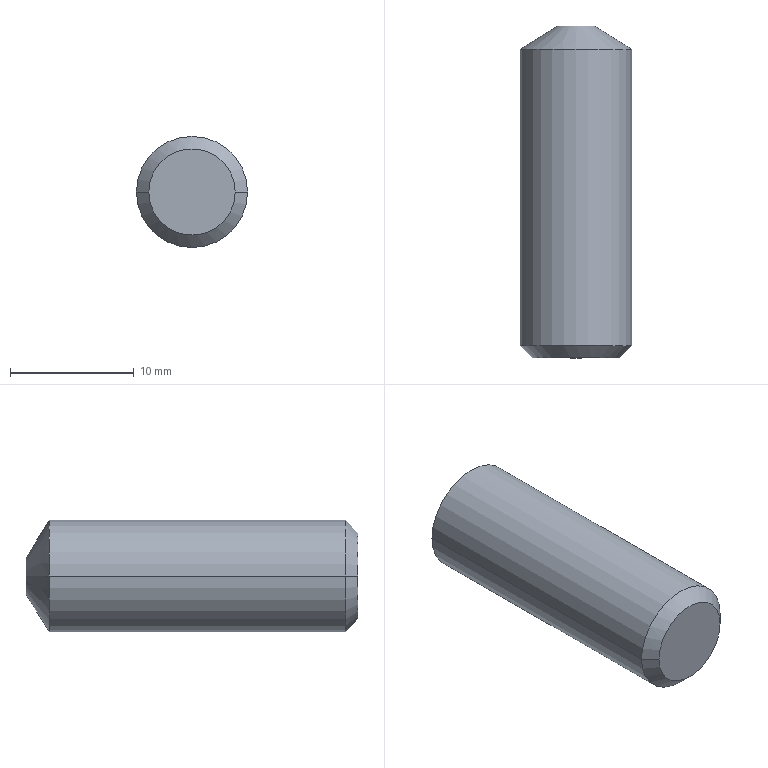Part | SolidWorks | features Chamfer 1, Revolution 1 | 1 solid | 8 faces | box 9 x 26.875 x 9 mm | volume 1635 mm3 | cone 4 | cylinder 2 | plane 2 | commonest cylinder face diameters 9 x2
STEP:
#1=CARTESIAN_POINT('',(3.5,0.,0.));
#2=VERTEX_POINT('',#1);
#3=CARTESIAN_POINT('',(-3.5,0.,0.));
#4=VERTEX_POINT('',#3);
#5=CARTESIAN_POINT('',(0.,0.,0.));
#6=DIRECTION('',(0.,-1.,0.));
#7=DIRECTION('',(1.,0.,0.));
#8=AXIS2_PLACEMENT_3D('',#5,#6,#7);
#9=CIRCLE('',#8,3.5);
#10=EDGE_CURVE('',#2,#4,#9,.T.);
#11=ORIENTED_EDGE('',*,*,#10,.F.);
#12=CARTESIAN_POINT('',(4.5,1.,0.));
#13=VERTEX_POINT('',#12);
#14=CARTESIAN_POINT('',(3.5,0.,0.));
#15=DIRECTION('',(0.7071,0.7071,0.));
#16=VECTOR('',#15,1000.);
#17=LINE('',#14,#16);
#18=EDGE_CURVE('',#2,#13,#17,.T.);
#19=ORIENTED_EDGE('',*,*,#18,.T.);
#20=CARTESIAN_POINT('',(-4.5,1.,0.));
#21=VERTEX_POINT('',#20);
#22=CARTESIAN_POINT('',(0.,1.,0.));
#23=DIRECTION('',(0.,1.,0.));
#24=DIRECTION('',(1.,0.,0.));
#25=AXIS2_PLACEMENT_3D('',#22,#23,#24);
#26=CIRCLE('',#25,4.5);
#27=EDGE_CURVE('',#21,#13,#26,.T.);
#28=ORIENTED_EDGE('',*,*,#27,.F.);
#29=CARTESIAN_POINT('',(-3.5,0.,0.));
#30=DIRECTION('',(-0.7071,0.7071,0.));
#31=VECTOR('',#30,1000.);
#32=LINE('',#29,#31);
#33=EDGE_CURVE('',#4,#21,#32,.T.);
#34=ORIENTED_EDGE('',*,*,#33,.F.);
#35=EDGE_LOOP('',(#11,#19,#28,#34));
#36=FACE_OUTER_BOUND('',#35,.T.);
#37=CARTESIAN_POINT('',(0.,0.,0.));
#38=DIRECTION('',(0.,1.,0.));
#39=DIRECTION('',(-1.,0.,0.));
#40=AXIS2_PLACEMENT_3D('',#37,#38,#39);
#41=CONICAL_SURFACE('',#40,3.5,0.7854);
#42=ADVANCED_FACE('',(#36),#41,.T.);
#43=CARTESIAN_POINT('',(4.5,25.,0.));
#44=VERTEX_POINT('',#43);
#45=CARTESIAN_POINT('',(-4.5,25.,0.));
#46=VERTEX_POINT('',#45);
#47=CARTESIAN_POINT('',(0.,25.,0.));
#48=DIRECTION('',(0.,-1.,0.));
#49=DIRECTION('',(1.,0.,0.));
#50=AXIS2_PLACEMENT_3D('',#47,#48,#49);
#51=CIRCLE('',#50,4.5);
#52=EDGE_CURVE('',#44,#46,#51,.T.);
#53=ORIENTED_EDGE('',*,*,#52,.T.);
#54=CARTESIAN_POINT('',(-4.5,0.,0.));
#55=DIRECTION('',(0.,-1.,0.));
#56=VECTOR('',#55,1000.);
#57=LINE('',#54,#56);
#58=EDGE_CURVE('',#46,#21,#57,.T.);
#59=ORIENTED_EDGE('',*,*,#58,.T.);
#60=ORIENTED_EDGE('',*,*,#27,.T.);
#61=CARTESIAN_POINT('',(4.5,0.,0.));
#62=DIRECTION('',(0.,-1.,0.));
#63=VECTOR('',#62,1000.);
#64=LINE('',#61,#63);
#65=EDGE_CURVE('',#44,#13,#64,.T.);
#66=ORIENTED_EDGE('',*,*,#65,.F.);
#67=EDGE_LOOP('',(#53,#59,#60,#66));
#68=FACE_OUTER_BOUND('',#67,.T.);
#69=CARTESIAN_POINT('',(0.,0.,0.));
#70=DIRECTION('',(0.,-1.,0.));
#71=DIRECTION('',(1.,0.,0.));
#72=AXIS2_PLACEMENT_3D('',#69,#70,#71);
#73=CYLINDRICAL_SURFACE('',#72,4.5);
#74=ADVANCED_FACE('',(#68),#73,.T.);
#75=CARTESIAN_POINT('',(1.5,26.875,0.));
#76=VERTEX_POINT('',#75);
#77=CARTESIAN_POINT('',(-1.5,26.875,0.));
#78=VERTEX_POINT('',#77);
#79=CARTESIAN_POINT('',(0.,26.875,0.));
#80=DIRECTION('',(0.,-1.,0.));
#81=DIRECTION('',(1.,0.,0.));
#82=AXIS2_PLACEMENT_3D('',#79,#80,#81);
#83=CIRCLE('',#82,1.5);
#84=EDGE_CURVE('',#76,#78,#83,.T.);
#85=ORIENTED_EDGE('',*,*,#84,.T.);
#86=CARTESIAN_POINT('',(-4.5,25.,0.));
#87=DIRECTION('',(-0.848,-0.5299,0.));
#88=VECTOR('',#87,1000.);
#89=LINE('',#86,#88);
#90=EDGE_CURVE('',#78,#46,#89,.T.);
#91=ORIENTED_EDGE('',*,*,#90,.T.);
#92=ORIENTED_EDGE('',*,*,#52,.F.);
#93=CARTESIAN_POINT('',(4.5,25.,0.));
#94=DIRECTION('',(0.848,-0.5299,0.));
#95=VECTOR('',#94,1000.);
#96=LINE('',#93,#95);
#97=EDGE_CURVE('',#76,#44,#96,.T.);
#98=ORIENTED_EDGE('',*,*,#97,.F.);
#99=EDGE_LOOP('',(#85,#91,#92,#98));
#100=FACE_OUTER_BOUND('',#99,.T.);
#101=CARTESIAN_POINT('',(0.,25.,0.));
#102=DIRECTION('',(0.,-1.,0.));
#103=DIRECTION('',(1.,0.,0.));
#104=AXIS2_PLACEMENT_3D('',#101,#102,#103);
#105=CONICAL_SURFACE('',#104,4.5,1.012);
#106=ADVANCED_FACE('',(#100),#105,.T.);
#107=ORIENTED_EDGE('',*,*,#84,.F.);
#108=CARTESIAN_POINT('',(0.,26.875,0.));
#109=DIRECTION('',(0.,-1.,0.));
#110=DIRECTION('',(1.,0.,0.));
#111=AXIS2_PLACEMENT_3D('',#108,#109,#110);
#112=CIRCLE('',#111,1.5);
#113=EDGE_CURVE('',#78,#76,#112,.T.);
#114=ORIENTED_EDGE('',*,*,#113,.F.);
#115=EDGE_LOOP('',(#107,#114));
#116=FACE_OUTER_BOUND('',#115,.T.);
#117=CARTESIAN_POINT('',(0.,26.875,0.));
#118=DIRECTION('',(0.,1.,0.));
#119=DIRECTION('',(-1.,0.,0.));
#120=AXIS2_PLACEMENT_3D('',#117,#118,#119);
#121=PLANE('',#120);
#122=ADVANCED_FACE('',(#116),#121,.T.);
#123=ORIENTED_EDGE('',*,*,#90,.F.);
#124=ORIENTED_EDGE('',*,*,#113,.T.);
#125=ORIENTED_EDGE('',*,*,#97,.T.);
#126=CARTESIAN_POINT('',(0.,25.,0.));
#127=DIRECTION('',(0.,-1.,0.));
#128=DIRECTION('',(1.,0.,0.));
#129=AXIS2_PLACEMENT_3D('',#126,#127,#128);
#130=CIRCLE('',#129,4.5);
#131=EDGE_CURVE('',#46,#44,#130,.T.);
#132=ORIENTED_EDGE('',*,*,#131,.F.);
#133=EDGE_LOOP('',(#123,#124,#125,#132));
#134=FACE_OUTER_BOUND('',#133,.T.);
#135=CARTESIAN_POINT('',(0.,25.,0.));
#136=DIRECTION('',(0.,-1.,0.));
#137=DIRECTION('',(1.,0.,0.));
#138=AXIS2_PLACEMENT_3D('',#135,#136,#137);
#139=CONICAL_SURFACE('',#138,4.5,1.012);
#140=ADVANCED_FACE('',(#134),#139,.T.);
#141=ORIENTED_EDGE('',*,*,#58,.F.);
#142=ORIENTED_EDGE('',*,*,#131,.T.);
#143=ORIENTED_EDGE('',*,*,#65,.T.);
#144=CARTESIAN_POINT('',(0.,1.,0.));
#145=DIRECTION('',(0.,1.,0.));
#146=DIRECTION('',(1.,0.,0.));
#147=AXIS2_PLACEMENT_3D('',#144,#145,#146);
#148=CIRCLE('',#147,4.5);
#149=EDGE_CURVE('',#13,#21,#148,.T.);
#150=ORIENTED_EDGE('',*,*,#149,.T.);
#151=EDGE_LOOP('',(#141,#142,#143,#150));
#152=FACE_OUTER_BOUND('',#151,.T.);
#153=CARTESIAN_POINT('',(0.,0.,0.));
#154=DIRECTION('',(0.,-1.,0.));
#155=DIRECTION('',(1.,0.,0.));
#156=AXIS2_PLACEMENT_3D('',#153,#154,#155);
#157=CYLINDRICAL_SURFACE('',#156,4.5);
#158=ADVANCED_FACE('',(#152),#157,.T.);
#159=CARTESIAN_POINT('',(0.,0.,0.));
#160=DIRECTION('',(0.,-1.,0.));
#161=DIRECTION('',(1.,0.,0.));
#162=AXIS2_PLACEMENT_3D('',#159,#160,#161);
#163=CIRCLE('',#162,3.5);
#164=EDGE_CURVE('',#4,#2,#163,.T.);
#165=ORIENTED_EDGE('',*,*,#164,.T.);
#166=ORIENTED_EDGE('',*,*,#10,.T.);
#167=EDGE_LOOP('',(#165,#166));
#168=FACE_OUTER_BOUND('',#167,.T.);
#169=CARTESIAN_POINT('',(4.5,0.,0.));
#170=DIRECTION('',(0.,-1.,0.));
#171=DIRECTION('',(1.,0.,0.));
#172=AXIS2_PLACEMENT_3D('',#169,#170,#171);
#173=PLANE('',#172);
#174=ADVANCED_FACE('',(#168),#173,.T.);
#175=ORIENTED_EDGE('',*,*,#18,.F.);
#176=ORIENTED_EDGE('',*,*,#164,.F.);
#177=ORIENTED_EDGE('',*,*,#33,.T.);
#178=ORIENTED_EDGE('',*,*,#149,.F.);
#179=EDGE_LOOP('',(#175,#176,#177,#178));
#180=FACE_OUTER_BOUND('',#179,.T.);
#181=CARTESIAN_POINT('',(0.,0.,0.));
#182=DIRECTION('',(0.,1.,0.));
#183=DIRECTION('',(-1.,0.,0.));
#184=AXIS2_PLACEMENT_3D('',#181,#182,#183);
#185=CONICAL_SURFACE('',#184,3.5,0.7854);
#186=ADVANCED_FACE('',(#180),#185,.T.);
#187=CLOSED_SHELL('',(#42,#74,#106,#122,#140,#158,#174,#186));
#188=MANIFOLD_SOLID_BREP('',#187);
#189=CARTESIAN_POINT('',(0.,0.,0.));
#190=DIRECTION('',(0.,0.,1.));
#191=DIRECTION('',(1.,0.,0.));
#192=AXIS2_PLACEMENT_3D('',#189,#190,#191);
#193=(LENGTH_UNIT()NAMED_UNIT(*)SI_UNIT(.MILLI.,.METRE.));
#194=UNCERTAINTY_MEASURE_WITH_UNIT(LENGTH_MEASURE(0.00001),#193,'','');
#195=(NAMED_UNIT(*)PLANE_ANGLE_UNIT()SI_UNIT($,.RADIAN.));
#196=(NAMED_UNIT(*)SI_UNIT($,.STERADIAN.)SOLID_ANGLE_UNIT());
#197=(GEOMETRIC_REPRESENTATION_CONTEXT(3)GLOBAL_UNCERTAINTY_ASSIGNED_CONTEXT((#194))GLOBAL_UNIT_ASSIGNED_CONTEXT((#193,#195,#196))REPRESENTATION_CONTEXT('',''));
#198=ADVANCED_BREP_SHAPE_REPRESENTATION('',(#188,#192),#197);